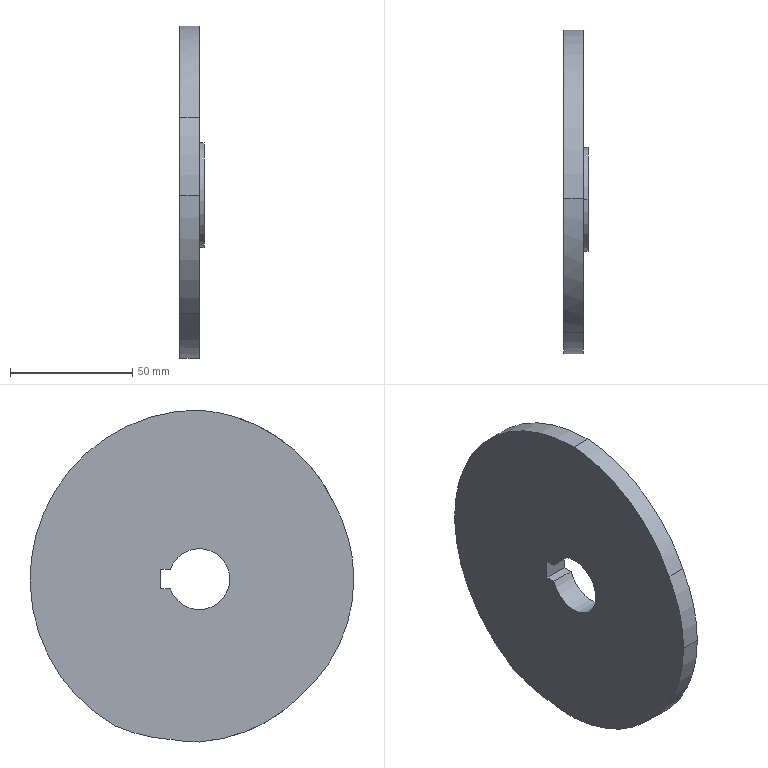Part | NX | 1 solid | 17 faces | box 10 x 132.62 x 136.02 mm | volume 110203 mm3 | cylinder 9 | plane 6 | spline 2 | commonest cylinder face diameters 25 x2 43 x2 126.62 x2 133.42 x1 135.238 x1 138.62 x1
STEP:
#1=CARTESIAN_POINT('',(-4.,-54.828,31.655));
#2=VERTEX_POINT('',#1);
#3=CARTESIAN_POINT('',(-4.,-63.31,0.));
#4=VERTEX_POINT('',#3);
#5=CARTESIAN_POINT('',(-4.,0.,0.));
#6=DIRECTION('',(1.,0.,0.));
#7=DIRECTION('',(0.,0.,-1.));
#8=AXIS2_PLACEMENT_3D('',#5,#6,#7);
#9=CIRCLE('',#8,63.31);
#10=EDGE_CURVE('',#2,#4,#9,.T.);
#11=ORIENTED_EDGE('',*,*,#10,.F.);
#12=CARTESIAN_POINT('',(-4.,0.000000957,69.31));
#13=VERTEX_POINT('',#12);
#14=CARTESIAN_POINT('',(-4.,-54.828,31.655));
#15=CARTESIAN_POINT('',(-4.,-52.486,36.717));
#16=CARTESIAN_POINT('',(-4.,-46.452,46.246));
#17=CARTESIAN_POINT('',(-4.,-29.392,61.957));
#18=CARTESIAN_POINT('',(-4.,-12.082,68.311));
#19=CARTESIAN_POINT('',(-4.,0.,69.31));
#20=B_SPLINE_CURVE_WITH_KNOTS('',3,(#14,#15,#16,#17,#18,#19),.UNSPECIFIED.,.F.,.F.,(4,1,1,4),(0.000000002,0.25,0.5,1.),.UNSPECIFIED.);
#21=EDGE_CURVE('',#13,#2,#20,.F.);
#22=ORIENTED_EDGE('',*,*,#21,.F.);
#23=CARTESIAN_POINT('',(-4.,34.656,-60.023));
#24=VERTEX_POINT('',#23);
#25=CARTESIAN_POINT('',(-4.,0.,0.));
#26=DIRECTION('',(1.,0.,0.));
#27=DIRECTION('',(0.,0.5,-0.866));
#28=AXIS2_PLACEMENT_3D('',#25,#26,#27);
#29=CIRCLE('',#28,69.31);
#30=EDGE_CURVE('',#24,#13,#29,.T.);
#31=ORIENTED_EDGE('',*,*,#30,.F.);
#32=CARTESIAN_POINT('',(-4.,11.584,-65.697));
#33=VERTEX_POINT('',#32);
#34=CARTESIAN_POINT('',(-4.,7.223,1.781));
#35=DIRECTION('',(1.,0.000000006,-0.000000023));
#36=DIRECTION('',(-0.000000023,0.0645,-0.9979));
#37=AXIS2_PLACEMENT_3D('',#34,#35,#36);
#38=CIRCLE('',#37,67.619);
#39=EDGE_CURVE('',#33,#24,#38,.T.);
#40=ORIENTED_EDGE('',*,*,#39,.F.);
#41=CARTESIAN_POINT('',(-4.,0.000000396,-66.71));
#42=VERTEX_POINT('',#41);
#43=CARTESIAN_POINT('',(-4.,0.,0.));
#44=DIRECTION('',(1.,0.,0.));
#45=DIRECTION('',(0.,0.,-1.));
#46=AXIS2_PLACEMENT_3D('',#43,#44,#45);
#47=CIRCLE('',#46,66.71);
#48=EDGE_CURVE('',#42,#33,#47,.T.);
#49=ORIENTED_EDGE('',*,*,#48,.F.);
#50=CARTESIAN_POINT('',(-4.,-40.695,-48.498));
#51=VERTEX_POINT('',#50);
#52=CARTESIAN_POINT('',(-4.,0.,-66.71));
#53=CARTESIAN_POINT('',(-4.,-7.747,-66.144));
#54=CARTESIAN_POINT('',(-4.,-22.895,-62.266));
#55=CARTESIAN_POINT('',(-4.,-35.402,-53.681));
#56=CARTESIAN_POINT('',(-4.,-40.695,-48.498));
#57=B_SPLINE_CURVE_WITH_KNOTS('',3,(#52,#53,#54,#55,#56),.UNSPECIFIED.,.F.,.F.,(4,1,4),(0.,0.5,1.),.UNSPECIFIED.);
#58=EDGE_CURVE('',#51,#42,#57,.F.);
#59=ORIENTED_EDGE('',*,*,#58,.F.);
#60=CARTESIAN_POINT('',(-4.,0.,0.));
#61=DIRECTION('',(1.,0.,0.));
#62=DIRECTION('',(0.,0.,-1.));
#63=AXIS2_PLACEMENT_3D('',#60,#61,#62);
#64=CIRCLE('',#63,63.31);
#65=EDGE_CURVE('',#4,#51,#64,.T.);
#66=ORIENTED_EDGE('',*,*,#65,.F.);
#67=EDGE_LOOP('',(#11,#22,#31,#40,#49,#59,#66));
#68=FACE_BOUND('',#67,.T.);
#69=CARTESIAN_POINT('',(-4.,15.8,4.));
#70=VERTEX_POINT('',#69);
#71=CARTESIAN_POINT('',(-4.,11.843,4.));
#72=VERTEX_POINT('',#71);
#73=CARTESIAN_POINT('',(-4.,15.8,4.));
#74=DIRECTION('',(0.,-1.,0.));
#75=VECTOR('',#74,1000.);
#76=LINE('',#73,#75);
#77=EDGE_CURVE('',#70,#72,#76,.T.);
#78=ORIENTED_EDGE('',*,*,#77,.T.);
#79=CARTESIAN_POINT('',(-4.,-12.5,0.));
#80=VERTEX_POINT('',#79);
#81=CARTESIAN_POINT('',(-4.,0.,0.));
#82=DIRECTION('',(-1.,0.,0.));
#83=DIRECTION('',(0.,-1.,0.));
#84=AXIS2_PLACEMENT_3D('',#81,#82,#83);
#85=CIRCLE('',#84,12.5);
#86=EDGE_CURVE('',#80,#72,#85,.T.);
#87=ORIENTED_EDGE('',*,*,#86,.F.);
#88=CARTESIAN_POINT('',(-4.,11.843,-4.));
#89=VERTEX_POINT('',#88);
#90=CARTESIAN_POINT('',(-4.,0.,0.));
#91=DIRECTION('',(-1.,0.,0.));
#92=DIRECTION('',(0.,-1.,0.));
#93=AXIS2_PLACEMENT_3D('',#90,#91,#92);
#94=CIRCLE('',#93,12.5);
#95=EDGE_CURVE('',#89,#80,#94,.T.);
#96=ORIENTED_EDGE('',*,*,#95,.F.);
#97=CARTESIAN_POINT('',(-4.,15.8,-4.));
#98=VERTEX_POINT('',#97);
#99=CARTESIAN_POINT('',(-4.,11.843,-4.));
#100=DIRECTION('',(0.,1.,0.));
#101=VECTOR('',#100,1000.);
#102=LINE('',#99,#101);
#103=EDGE_CURVE('',#89,#98,#102,.T.);
#104=ORIENTED_EDGE('',*,*,#103,.T.);
#105=CARTESIAN_POINT('',(-4.,15.8,-4.));
#106=DIRECTION('',(0.,0.,1.));
#107=VECTOR('',#106,1000.);
#108=LINE('',#105,#107);
#109=EDGE_CURVE('',#98,#70,#108,.T.);
#110=ORIENTED_EDGE('',*,*,#109,.T.);
#111=EDGE_LOOP('',(#78,#87,#96,#104,#110));
#112=FACE_BOUND('',#111,.T.);
#113=CARTESIAN_POINT('',(-4.,0.,0.));
#114=DIRECTION('',(1.,0.,0.));
#115=DIRECTION('',(0.,1.,0.));
#116=AXIS2_PLACEMENT_3D('',#113,#114,#115);
#117=PLANE('',#116);
#118=ADVANCED_FACE('',(#68,#112),#117,.F.);
#119=CARTESIAN_POINT('',(4.,-63.31,0.));
#120=VERTEX_POINT('',#119);
#121=CARTESIAN_POINT('',(4.,-63.31,0.));
#122=DIRECTION('',(1.,0.,0.));
#123=VECTOR('',#122,1000.);
#124=LINE('',#121,#123);
#125=EDGE_CURVE('',#4,#120,#124,.T.);
#126=ORIENTED_EDGE('',*,*,#125,.F.);
#127=ORIENTED_EDGE('',*,*,#65,.T.);
#128=CARTESIAN_POINT('',(4.,-40.695,-48.498));
#129=VERTEX_POINT('',#128);
#130=CARTESIAN_POINT('',(2.094,-40.695,-48.498));
#131=DIRECTION('',(1.,0.,0.));
#132=VECTOR('',#131,1000.);
#133=LINE('',#130,#132);
#134=EDGE_CURVE('',#51,#129,#133,.T.);
#135=ORIENTED_EDGE('',*,*,#134,.T.);
#136=CARTESIAN_POINT('',(4.,0.,0.));
#137=DIRECTION('',(-1.,0.,0.));
#138=DIRECTION('',(0.,0.,-1.));
#139=AXIS2_PLACEMENT_3D('',#136,#137,#138);
#140=CIRCLE('',#139,63.31);
#141=EDGE_CURVE('',#129,#120,#140,.T.);
#142=ORIENTED_EDGE('',*,*,#141,.T.);
#143=EDGE_LOOP('',(#126,#127,#135,#142));
#144=FACE_BOUND('',#143,.T.);
#145=CARTESIAN_POINT('',(4.,0.,0.));
#146=DIRECTION('',(1.,0.,0.));
#147=DIRECTION('',(0.,-1.,0.));
#148=AXIS2_PLACEMENT_3D('',#145,#146,#147);
#149=CYLINDRICAL_SURFACE('',#148,63.31);
#150=ADVANCED_FACE('',(#144),#149,.T.);
#151=CARTESIAN_POINT('',(4.,0.000001163,69.31));
#152=VERTEX_POINT('',#151);
#153=CARTESIAN_POINT('',(-4.,0.,69.31));
#154=CARTESIAN_POINT('',(-1.333,0.000000217,69.31));
#155=CARTESIAN_POINT('',(1.333,0.000000434,69.31));
#156=CARTESIAN_POINT('',(4.,0.00000065,69.31));
#157=B_SPLINE_CURVE_WITH_KNOTS('',3,(#153,#154,#155,#156),.UNSPECIFIED.,.F.,.F.,(4,4),(0.,1.),.UNSPECIFIED.);
#158=EDGE_CURVE('',#13,#152,#157,.T.);
#159=ORIENTED_EDGE('',*,*,#158,.F.);
#160=ORIENTED_EDGE('',*,*,#21,.T.);
#161=CARTESIAN_POINT('',(4.,-54.828,31.655));
#162=VERTEX_POINT('',#161);
#163=CARTESIAN_POINT('',(4.,-54.828,31.655));
#164=CARTESIAN_POINT('',(1.333,-54.828,31.655));
#165=CARTESIAN_POINT('',(-1.333,-54.828,31.655));
#166=CARTESIAN_POINT('',(-4.,-54.828,31.655));
#167=B_SPLINE_CURVE_WITH_KNOTS('',3,(#163,#164,#165,#166),.UNSPECIFIED.,.F.,.F.,(4,4),(0.,1.),.UNSPECIFIED.);
#168=EDGE_CURVE('',#162,#2,#167,.T.);
#169=ORIENTED_EDGE('',*,*,#168,.F.);
#170=CARTESIAN_POINT('',(4.,0.00000065,69.31));
#171=CARTESIAN_POINT('',(4.,-3.02,69.013));
#172=CARTESIAN_POINT('',(4.,-9.009,68.185));
#173=CARTESIAN_POINT('',(4.,-20.507,64.838));
#174=CARTESIAN_POINT('',(4.,-33.649,58.028));
#175=CARTESIAN_POINT('',(4.,-46.454,46.246));
#176=CARTESIAN_POINT('',(4.,-52.485,36.718));
#177=CARTESIAN_POINT('',(4.,-54.828,31.655));
#178=B_SPLINE_CURVE_WITH_KNOTS('',3,(#170,#171,#172,#173,#174,#175,#176,#177),.UNSPECIFIED.,.F.,.F.,(4,1,1,1,1,4),(0.,0.125,0.25,0.5,0.75,1.),.UNSPECIFIED.);
#179=EDGE_CURVE('',#162,#152,#178,.F.);
#180=ORIENTED_EDGE('',*,*,#179,.T.);
#181=EDGE_LOOP('',(#159,#160,#169,#180));
#182=FACE_BOUND('',#181,.T.);
#183=CARTESIAN_POINT('',(4.,0.000001951,69.31));
#184=CARTESIAN_POINT('',(-4.,0.000001951,69.31));
#185=CARTESIAN_POINT('',(4.,-12.097,68.31));
#186=CARTESIAN_POINT('',(-4.,-12.097,68.31));
#187=CARTESIAN_POINT('',(4.,-35.177,59.835));
#188=CARTESIAN_POINT('',(-4.,-35.177,59.835));
#189=CARTESIAN_POINT('',(4.,-50.169,41.724));
#190=CARTESIAN_POINT('',(-4.,-50.169,41.724));
#191=CARTESIAN_POINT('',(4.,-54.828,31.655));
#192=CARTESIAN_POINT('',(-4.,-54.828,31.655));
#193=B_SPLINE_SURFACE_WITH_KNOTS('',3,1,((#183,#184),(#185,#186),(#187,#188),(#189,#190),(#191,#192)),.SURF_OF_LINEAR_EXTRUSION.,.F.,.F.,.F.,(4,1,4),(2,2),(0.009378,0.4996,0.9897),(0.,1.),.UNSPECIFIED.);
#194=ADVANCED_FACE('',(#182),#193,.F.);
#195=CARTESIAN_POINT('',(4.,34.656,-60.023));
#196=VERTEX_POINT('',#195);
#197=CARTESIAN_POINT('',(4.,0.,0.));
#198=DIRECTION('',(-1.,0.,0.));
#199=DIRECTION('',(0.,0.,1.));
#200=AXIS2_PLACEMENT_3D('',#197,#198,#199);
#201=CIRCLE('',#200,69.31);
#202=EDGE_CURVE('',#152,#196,#201,.T.);
#203=ORIENTED_EDGE('',*,*,#202,.T.);
#204=CARTESIAN_POINT('',(4.,34.657,-60.023));
#205=CARTESIAN_POINT('',(1.333,34.657,-60.023));
#206=CARTESIAN_POINT('',(-1.333,34.657,-60.023));
#207=CARTESIAN_POINT('',(-4.,34.657,-60.023));
#208=B_SPLINE_CURVE_WITH_KNOTS('',3,(#204,#205,#206,#207),.UNSPECIFIED.,.F.,.F.,(4,4),(0.,1.),.UNSPECIFIED.);
#209=EDGE_CURVE('',#196,#24,#208,.T.);
#210=ORIENTED_EDGE('',*,*,#209,.T.);
#211=ORIENTED_EDGE('',*,*,#30,.T.);
#212=ORIENTED_EDGE('',*,*,#158,.T.);
#213=EDGE_LOOP('',(#203,#210,#211,#212));
#214=FACE_BOUND('',#213,.T.);
#215=CARTESIAN_POINT('',(4.,0.,0.));
#216=DIRECTION('',(1.,0.,0.));
#217=DIRECTION('',(0.,0.5,-0.866));
#218=AXIS2_PLACEMENT_3D('',#215,#216,#217);
#219=CYLINDRICAL_SURFACE('',#218,69.31);
#220=ADVANCED_FACE('',(#214),#219,.T.);
#221=ORIENTED_EDGE('',*,*,#141,.F.);
#222=CARTESIAN_POINT('',(4.,0.000000396,-66.71));
#223=VERTEX_POINT('',#222);
#224=CARTESIAN_POINT('',(4.,-40.695,-48.498));
#225=CARTESIAN_POINT('',(4.,-35.403,-53.68));
#226=CARTESIAN_POINT('',(4.,-22.893,-62.267));
#227=CARTESIAN_POINT('',(4.,-7.749,-66.144));
#228=CARTESIAN_POINT('',(4.,0.,-66.71));
#229=B_SPLINE_CURVE_WITH_KNOTS('',3,(#224,#225,#226,#227,#228),.UNSPECIFIED.,.F.,.F.,(4,1,4),(0.000002282,0.5,1.),.UNSPECIFIED.);
#230=EDGE_CURVE('',#223,#129,#229,.F.);
#231=ORIENTED_EDGE('',*,*,#230,.F.);
#232=CARTESIAN_POINT('',(4.,11.584,-65.697));
#233=VERTEX_POINT('',#232);
#234=CARTESIAN_POINT('',(4.,0.,0.));
#235=DIRECTION('',(-1.,0.,0.));
#236=DIRECTION('',(0.,0.1736,-0.9848));
#237=AXIS2_PLACEMENT_3D('',#234,#235,#236);
#238=CIRCLE('',#237,66.71);
#239=EDGE_CURVE('',#233,#223,#238,.T.);
#240=ORIENTED_EDGE('',*,*,#239,.F.);
#241=CARTESIAN_POINT('',(4.,7.223,1.781));
#242=DIRECTION('',(-1.,-0.000000006,0.000000023));
#243=DIRECTION('',(-0.000000023,0.4057,-0.914));
#244=AXIS2_PLACEMENT_3D('',#241,#242,#243);
#245=CIRCLE('',#244,67.619);
#246=EDGE_CURVE('',#196,#233,#245,.T.);
#247=ORIENTED_EDGE('',*,*,#246,.F.);
#248=ORIENTED_EDGE('',*,*,#202,.F.);
#249=ORIENTED_EDGE('',*,*,#179,.F.);
#250=CARTESIAN_POINT('',(4.,0.,0.));
#251=DIRECTION('',(-1.,0.,0.));
#252=DIRECTION('',(0.,0.,-1.));
#253=AXIS2_PLACEMENT_3D('',#250,#251,#252);
#254=CIRCLE('',#253,63.31);
#255=EDGE_CURVE('',#120,#162,#254,.T.);
#256=ORIENTED_EDGE('',*,*,#255,.F.);
#257=EDGE_LOOP('',(#221,#231,#240,#247,#248,#249,#256));
#258=FACE_BOUND('',#257,.T.);
#259=CARTESIAN_POINT('',(4.,0.,21.5));
#260=VERTEX_POINT('',#259);
#261=CARTESIAN_POINT('',(4.,0.,-21.5));
#262=VERTEX_POINT('',#261);
#263=CARTESIAN_POINT('',(4.,0.,0.));
#264=DIRECTION('',(1.,0.,0.));
#265=DIRECTION('',(0.,0.,1.));
#266=AXIS2_PLACEMENT_3D('',#263,#264,#265);
#267=CIRCLE('',#266,21.5);
#268=EDGE_CURVE('',#260,#262,#267,.T.);
#269=ORIENTED_EDGE('',*,*,#268,.F.);
#270=CARTESIAN_POINT('',(4.,0.,0.));
#271=DIRECTION('',(1.,0.,0.));
#272=DIRECTION('',(0.,0.,1.));
#273=AXIS2_PLACEMENT_3D('',#270,#271,#272);
#274=CIRCLE('',#273,21.5);
#275=EDGE_CURVE('',#262,#260,#274,.T.);
#276=ORIENTED_EDGE('',*,*,#275,.F.);
#277=EDGE_LOOP('',(#269,#276));
#278=FACE_BOUND('',#277,.T.);
#279=CARTESIAN_POINT('',(4.,0.,0.));
#280=DIRECTION('',(1.,0.,0.));
#281=DIRECTION('',(0.,1.,0.));
#282=AXIS2_PLACEMENT_3D('',#279,#280,#281);
#283=PLANE('',#282);
#284=ADVANCED_FACE('',(#258,#278),#283,.T.);
#285=CARTESIAN_POINT('',(4.,11.584,-65.697));
#286=CARTESIAN_POINT('',(1.333,11.584,-65.697));
#287=CARTESIAN_POINT('',(-1.333,11.584,-65.697));
#288=CARTESIAN_POINT('',(-4.,11.584,-65.697));
#289=B_SPLINE_CURVE_WITH_KNOTS('',3,(#285,#286,#287,#288),.UNSPECIFIED.,.F.,.F.,(4,4),(0.,1.),.UNSPECIFIED.);
#290=EDGE_CURVE('',#233,#33,#289,.T.);
#291=ORIENTED_EDGE('',*,*,#290,.T.);
#292=ORIENTED_EDGE('',*,*,#39,.T.);
#293=ORIENTED_EDGE('',*,*,#209,.F.);
#294=ORIENTED_EDGE('',*,*,#246,.T.);
#295=EDGE_LOOP('',(#291,#292,#293,#294));
#296=FACE_BOUND('',#295,.T.);
#297=CARTESIAN_POINT('',(0.,7.223,1.781));
#298=DIRECTION('',(-1.,-0.000000006,0.000000023));
#299=DIRECTION('',(-0.000000023,0.0645,-0.9979));
#300=AXIS2_PLACEMENT_3D('',#297,#298,#299);
#301=CYLINDRICAL_SURFACE('',#300,67.619);
#302=ADVANCED_FACE('',(#296),#301,.T.);
#303=CARTESIAN_POINT('',(4.,0.,-66.71));
#304=CARTESIAN_POINT('',(1.333,0.,-66.71));
#305=CARTESIAN_POINT('',(-1.333,0.,-66.71));
#306=CARTESIAN_POINT('',(-4.,0.,-66.71));
#307=B_SPLINE_CURVE_WITH_KNOTS('',3,(#303,#304,#305,#306),.UNSPECIFIED.,.F.,.F.,(4,4),(0.,1.),.UNSPECIFIED.);
#308=EDGE_CURVE('',#42,#223,#307,.F.);
#309=ORIENTED_EDGE('',*,*,#308,.F.);
#310=ORIENTED_EDGE('',*,*,#48,.T.);
#311=ORIENTED_EDGE('',*,*,#290,.F.);
#312=ORIENTED_EDGE('',*,*,#239,.T.);
#313=EDGE_LOOP('',(#309,#310,#311,#312));
#314=FACE_BOUND('',#313,.T.);
#315=CARTESIAN_POINT('',(4.,0.,0.));
#316=DIRECTION('',(1.,0.,0.));
#317=DIRECTION('',(0.,0.,-1.));
#318=AXIS2_PLACEMENT_3D('',#315,#316,#317);
#319=CYLINDRICAL_SURFACE('',#318,66.71);
#320=ADVANCED_FACE('',(#314),#319,.T.);
#321=ORIENTED_EDGE('',*,*,#134,.F.);
#322=ORIENTED_EDGE('',*,*,#58,.T.);
#323=ORIENTED_EDGE('',*,*,#308,.T.);
#324=ORIENTED_EDGE('',*,*,#230,.T.);
#325=EDGE_LOOP('',(#321,#322,#323,#324));
#326=FACE_BOUND('',#325,.T.);
#327=CARTESIAN_POINT('',(4.,-40.885,-48.312));
#328=CARTESIAN_POINT('',(-4.,-40.885,-48.312));
#329=CARTESIAN_POINT('',(4.,-35.574,-53.512));
#330=CARTESIAN_POINT('',(-4.,-35.574,-53.512));
#331=CARTESIAN_POINT('',(4.,-23.027,-62.24));
#332=CARTESIAN_POINT('',(-4.,-23.027,-62.24));
#333=CARTESIAN_POINT('',(4.,-7.809,-66.14));
#334=CARTESIAN_POINT('',(-4.,-7.809,-66.14));
#335=CARTESIAN_POINT('',(4.,0.000000816,-66.71));
#336=CARTESIAN_POINT('',(-4.,0.000000816,-66.71));
#337=B_SPLINE_SURFACE_WITH_KNOTS('',3,1,((#327,#328),(#329,#330),(#331,#332),(#333,#334),(#335,#336)),.SURF_OF_LINEAR_EXTRUSION.,.F.,.F.,.F.,(4,1,4),(2,2),(0.004188,0.4973,0.9904),(0.,1.),.UNSPECIFIED.);
#338=ADVANCED_FACE('',(#326),#337,.F.);
#339=CARTESIAN_POINT('',(6.,0.,-21.5));
#340=VERTEX_POINT('',#339);
#341=CARTESIAN_POINT('',(6.,0.,21.5));
#342=VERTEX_POINT('',#341);
#343=CARTESIAN_POINT('',(6.,0.,0.));
#344=DIRECTION('',(-1.,0.,0.));
#345=DIRECTION('',(0.,0.,1.));
#346=AXIS2_PLACEMENT_3D('',#343,#344,#345);
#347=CIRCLE('',#346,21.5);
#348=EDGE_CURVE('',#340,#342,#347,.T.);
#349=ORIENTED_EDGE('',*,*,#348,.T.);
#350=CARTESIAN_POINT('',(4.,0.,21.5));
#351=DIRECTION('',(-1.,0.,0.));
#352=VECTOR('',#351,1000.);
#353=LINE('',#350,#352);
#354=EDGE_CURVE('',#342,#260,#353,.T.);
#355=ORIENTED_EDGE('',*,*,#354,.T.);
#356=ORIENTED_EDGE('',*,*,#268,.T.);
#357=CARTESIAN_POINT('',(4.,0.,-21.5));
#358=DIRECTION('',(-1.,0.,0.));
#359=VECTOR('',#358,1000.);
#360=LINE('',#357,#359);
#361=EDGE_CURVE('',#340,#262,#360,.T.);
#362=ORIENTED_EDGE('',*,*,#361,.F.);
#363=EDGE_LOOP('',(#349,#355,#356,#362));
#364=FACE_BOUND('',#363,.T.);
#365=CARTESIAN_POINT('',(4.,0.,0.));
#366=DIRECTION('',(-1.,0.,0.));
#367=DIRECTION('',(0.,0.,1.));
#368=AXIS2_PLACEMENT_3D('',#365,#366,#367);
#369=CYLINDRICAL_SURFACE('',#368,21.5);
#370=ADVANCED_FACE('',(#364),#369,.T.);
#371=ORIENTED_EDGE('',*,*,#109,.F.);
#372=CARTESIAN_POINT('',(6.,15.8,-4.));
#373=VERTEX_POINT('',#372);
#374=CARTESIAN_POINT('',(6.,15.8,-4.));
#375=DIRECTION('',(-1.,0.,0.));
#376=VECTOR('',#375,1000.);
#377=LINE('',#374,#376);
#378=EDGE_CURVE('',#373,#98,#377,.T.);
#379=ORIENTED_EDGE('',*,*,#378,.F.);
#380=CARTESIAN_POINT('',(6.,15.8,4.));
#381=VERTEX_POINT('',#380);
#382=CARTESIAN_POINT('',(6.,15.8,-4.));
#383=DIRECTION('',(0.,0.,1.));
#384=VECTOR('',#383,1000.);
#385=LINE('',#382,#384);
#386=EDGE_CURVE('',#373,#381,#385,.T.);
#387=ORIENTED_EDGE('',*,*,#386,.T.);
#388=CARTESIAN_POINT('',(6.,15.8,4.));
#389=DIRECTION('',(-1.,0.,0.));
#390=VECTOR('',#389,1000.);
#391=LINE('',#388,#390);
#392=EDGE_CURVE('',#381,#70,#391,.T.);
#393=ORIENTED_EDGE('',*,*,#392,.T.);
#394=EDGE_LOOP('',(#371,#379,#387,#393));
#395=FACE_BOUND('',#394,.T.);
#396=CARTESIAN_POINT('',(-4.,15.8,4.));
#397=DIRECTION('',(0.,1.,0.));
#398=DIRECTION('',(1.,0.,0.));
#399=AXIS2_PLACEMENT_3D('',#396,#397,#398);
#400=PLANE('',#399);
#401=ADVANCED_FACE('',(#395),#400,.F.);
#402=ORIENTED_EDGE('',*,*,#348,.F.);
#403=CARTESIAN_POINT('',(6.,0.,0.));
#404=DIRECTION('',(-1.,0.,0.));
#405=DIRECTION('',(0.,0.,1.));
#406=AXIS2_PLACEMENT_3D('',#403,#404,#405);
#407=CIRCLE('',#406,21.5);
#408=EDGE_CURVE('',#342,#340,#407,.T.);
#409=ORIENTED_EDGE('',*,*,#408,.F.);
#410=EDGE_LOOP('',(#402,#409));
#411=FACE_BOUND('',#410,.T.);
#412=CARTESIAN_POINT('',(6.,11.843,4.));
#413=VERTEX_POINT('',#412);
#414=CARTESIAN_POINT('',(6.,15.8,4.));
#415=DIRECTION('',(0.,-1.,0.));
#416=VECTOR('',#415,1000.);
#417=LINE('',#414,#416);
#418=EDGE_CURVE('',#381,#413,#417,.T.);
#419=ORIENTED_EDGE('',*,*,#418,.F.);
#420=ORIENTED_EDGE('',*,*,#386,.F.);
#421=CARTESIAN_POINT('',(6.,11.843,-4.));
#422=VERTEX_POINT('',#421);
#423=CARTESIAN_POINT('',(6.,11.843,-4.));
#424=DIRECTION('',(0.,1.,0.));
#425=VECTOR('',#424,1000.);
#426=LINE('',#423,#425);
#427=EDGE_CURVE('',#422,#373,#426,.T.);
#428=ORIENTED_EDGE('',*,*,#427,.F.);
#429=CARTESIAN_POINT('',(6.,-12.5,0.));
#430=VERTEX_POINT('',#429);
#431=CARTESIAN_POINT('',(6.,0.,0.));
#432=DIRECTION('',(1.,0.,0.));
#433=DIRECTION('',(0.,-1.,0.));
#434=AXIS2_PLACEMENT_3D('',#431,#432,#433);
#435=CIRCLE('',#434,12.5);
#436=EDGE_CURVE('',#430,#422,#435,.T.);
#437=ORIENTED_EDGE('',*,*,#436,.F.);
#438=CARTESIAN_POINT('',(6.,0.,0.));
#439=DIRECTION('',(1.,0.,0.));
#440=DIRECTION('',(0.,-1.,0.));
#441=AXIS2_PLACEMENT_3D('',#438,#439,#440);
#442=CIRCLE('',#441,12.5);
#443=EDGE_CURVE('',#413,#430,#442,.T.);
#444=ORIENTED_EDGE('',*,*,#443,.F.);
#445=EDGE_LOOP('',(#419,#420,#428,#437,#444));
#446=FACE_BOUND('',#445,.T.);
#447=CARTESIAN_POINT('',(6.,0.,0.));
#448=DIRECTION('',(-1.,0.,0.));
#449=DIRECTION('',(0.,0.,1.));
#450=AXIS2_PLACEMENT_3D('',#447,#448,#449);
#451=PLANE('',#450);
#452=ADVANCED_FACE('',(#411,#446),#451,.F.);
#453=ORIENTED_EDGE('',*,*,#77,.F.);
#454=ORIENTED_EDGE('',*,*,#392,.F.);
#455=ORIENTED_EDGE('',*,*,#418,.T.);
#456=CARTESIAN_POINT('',(6.,11.843,4.));
#457=DIRECTION('',(-1.,0.,0.));
#458=VECTOR('',#457,1000.);
#459=LINE('',#456,#458);
#460=EDGE_CURVE('',#413,#72,#459,.T.);
#461=ORIENTED_EDGE('',*,*,#460,.T.);
#462=EDGE_LOOP('',(#453,#454,#455,#461));
#463=FACE_BOUND('',#462,.T.);
#464=CARTESIAN_POINT('',(-4.,11.843,4.));
#465=DIRECTION('',(0.,0.,1.));
#466=DIRECTION('',(1.,0.,0.));
#467=AXIS2_PLACEMENT_3D('',#464,#465,#466);
#468=PLANE('',#467);
#469=ADVANCED_FACE('',(#463),#468,.F.);
#470=CARTESIAN_POINT('',(-4.4,-12.5,0.));
#471=DIRECTION('',(1.,0.,0.));
#472=VECTOR('',#471,1000.);
#473=LINE('',#470,#472);
#474=EDGE_CURVE('',#80,#430,#473,.T.);
#475=ORIENTED_EDGE('',*,*,#474,.F.);
#476=ORIENTED_EDGE('',*,*,#86,.T.);
#477=ORIENTED_EDGE('',*,*,#460,.F.);
#478=ORIENTED_EDGE('',*,*,#443,.T.);
#479=EDGE_LOOP('',(#475,#476,#477,#478));
#480=FACE_BOUND('',#479,.T.);
#481=CARTESIAN_POINT('',(-4.4,0.,0.));
#482=DIRECTION('',(1.,0.,0.));
#483=DIRECTION('',(0.,-1.,0.));
#484=AXIS2_PLACEMENT_3D('',#481,#482,#483);
#485=CYLINDRICAL_SURFACE('',#484,12.5);
#486=ADVANCED_FACE('',(#480),#485,.F.);
#487=ORIENTED_EDGE('',*,*,#103,.F.);
#488=CARTESIAN_POINT('',(-4.,11.843,-4.));
#489=DIRECTION('',(1.,0.,0.));
#490=VECTOR('',#489,1000.);
#491=LINE('',#488,#490);
#492=EDGE_CURVE('',#89,#422,#491,.T.);
#493=ORIENTED_EDGE('',*,*,#492,.T.);
#494=ORIENTED_EDGE('',*,*,#427,.T.);
#495=ORIENTED_EDGE('',*,*,#378,.T.);
#496=EDGE_LOOP('',(#487,#493,#494,#495));
#497=FACE_BOUND('',#496,.T.);
#498=CARTESIAN_POINT('',(-4.,15.8,-4.));
#499=DIRECTION('',(0.,0.,-1.));
#500=DIRECTION('',(0.,-1.,0.));
#501=AXIS2_PLACEMENT_3D('',#498,#499,#500);
#502=PLANE('',#501);
#503=ADVANCED_FACE('',(#497),#502,.F.);
#504=ORIENTED_EDGE('',*,*,#354,.F.);
#505=ORIENTED_EDGE('',*,*,#408,.T.);
#506=ORIENTED_EDGE('',*,*,#361,.T.);
#507=ORIENTED_EDGE('',*,*,#275,.T.);
#508=EDGE_LOOP('',(#504,#505,#506,#507));
#509=FACE_BOUND('',#508,.T.);
#510=CARTESIAN_POINT('',(4.,0.,0.));
#511=DIRECTION('',(-1.,0.,0.));
#512=DIRECTION('',(0.,0.,1.));
#513=AXIS2_PLACEMENT_3D('',#510,#511,#512);
#514=CYLINDRICAL_SURFACE('',#513,21.5);
#515=ADVANCED_FACE('',(#509),#514,.T.);
#516=ORIENTED_EDGE('',*,*,#95,.T.);
#517=ORIENTED_EDGE('',*,*,#474,.T.);
#518=ORIENTED_EDGE('',*,*,#436,.T.);
#519=ORIENTED_EDGE('',*,*,#492,.F.);
#520=EDGE_LOOP('',(#516,#517,#518,#519));
#521=FACE_BOUND('',#520,.T.);
#522=CARTESIAN_POINT('',(-4.4,0.,0.));
#523=DIRECTION('',(1.,0.,0.));
#524=DIRECTION('',(0.,-1.,0.));
#525=AXIS2_PLACEMENT_3D('',#522,#523,#524);
#526=CYLINDRICAL_SURFACE('',#525,12.5);
#527=ADVANCED_FACE('',(#521),#526,.F.);
#528=ORIENTED_EDGE('',*,*,#10,.T.);
#529=ORIENTED_EDGE('',*,*,#125,.T.);
#530=ORIENTED_EDGE('',*,*,#255,.T.);
#531=ORIENTED_EDGE('',*,*,#168,.T.);
#532=EDGE_LOOP('',(#528,#529,#530,#531));
#533=FACE_BOUND('',#532,.T.);
#534=CARTESIAN_POINT('',(4.,0.,0.));
#535=DIRECTION('',(1.,0.,0.));
#536=DIRECTION('',(0.,-1.,0.));
#537=AXIS2_PLACEMENT_3D('',#534,#535,#536);
#538=CYLINDRICAL_SURFACE('',#537,63.31);
#539=ADVANCED_FACE('',(#533),#538,.T.);
#540=CLOSED_SHELL('',(#118,#150,#194,#220,#284,#302,#320,#338,#370,#401,#452,#469,#486,#503,#515,#527,#539));
#541=MANIFOLD_SOLID_BREP('',#540);
#542=(LENGTH_UNIT()NAMED_UNIT(*)SI_UNIT(.MILLI.,.METRE.));
#543=UNCERTAINTY_MEASURE_WITH_UNIT(LENGTH_MEASURE(0.0508),#542,'','');
#544=(NAMED_UNIT(*)PLANE_ANGLE_UNIT()SI_UNIT($,.RADIAN.));
#545=(NAMED_UNIT(*)SI_UNIT($,.STERADIAN.)SOLID_ANGLE_UNIT());
#546=(GEOMETRIC_REPRESENTATION_CONTEXT(3)GLOBAL_UNCERTAINTY_ASSIGNED_CONTEXT((#543))GLOBAL_UNIT_ASSIGNED_CONTEXT((#542,#544,#545))REPRESENTATION_CONTEXT('',''));
#547=ADVANCED_BREP_SHAPE_REPRESENTATION('',(#541),#546);